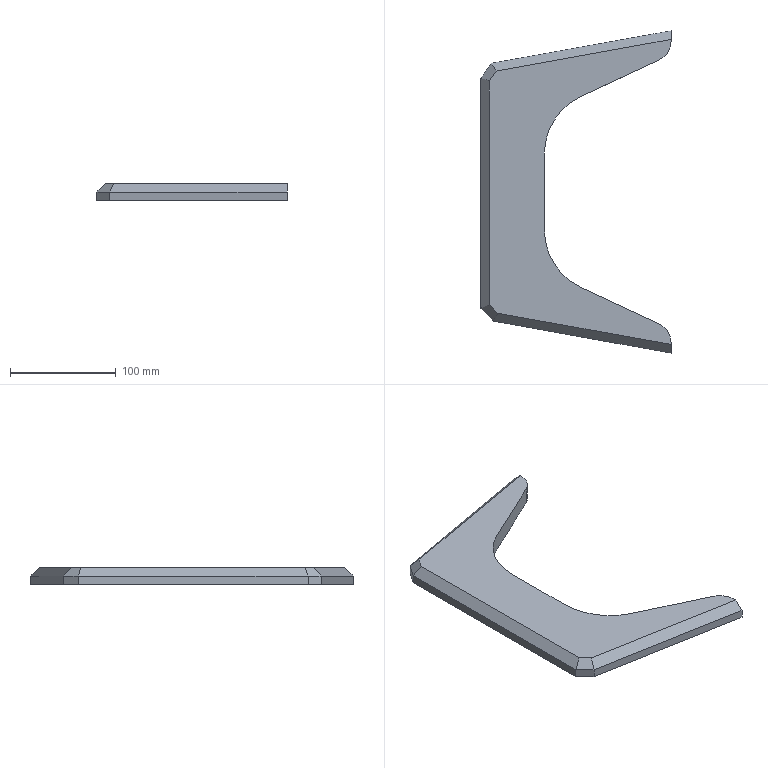Part | SolidWorks | features Chamfer 2, Extrusion 1 | 1 solid | 21 faces | box 180 x 305.1 x 16 mm | volume 379502 mm3 | plane 17 | cylinder 4 | commonest cylinder face diameters 40 x2 120 x2
STEP:
#1=CARTESIAN_POINT('',(9.84,121.779,0.));
#2=VERTEX_POINT('',#1);
#3=CARTESIAN_POINT('',(9.84,121.779,8.));
#4=VERTEX_POINT('',#3);
#5=CARTESIAN_POINT('',(9.84,121.779,16.));
#6=DIRECTION('',(0.,0.,1.));
#7=VECTOR('',#6,1000.);
#8=LINE('',#5,#7);
#9=EDGE_CURVE('',#2,#4,#8,.T.);
#10=ORIENTED_EDGE('',*,*,#9,.T.);
#11=CARTESIAN_POINT('',(180.,152.55,8.));
#12=VERTEX_POINT('',#11);
#13=CARTESIAN_POINT('',(0.,120.,8.));
#14=DIRECTION('',(0.984,0.1779,0.));
#15=VECTOR('',#14,1000.);
#16=LINE('',#13,#15);
#17=EDGE_CURVE('',#4,#12,#16,.T.);
#18=ORIENTED_EDGE('',*,*,#17,.T.);
#19=CARTESIAN_POINT('',(180.,152.55,0.));
#20=VERTEX_POINT('',#19);
#21=CARTESIAN_POINT('',(180.,152.55,16.));
#22=DIRECTION('',(0.,0.,-1.));
#23=VECTOR('',#22,1000.);
#24=LINE('',#21,#23);
#25=EDGE_CURVE('',#12,#20,#24,.T.);
#26=ORIENTED_EDGE('',*,*,#25,.T.);
#27=CARTESIAN_POINT('',(0.,120.,0.));
#28=DIRECTION('',(-0.984,-0.1779,0.));
#29=VECTOR('',#28,1000.);
#30=LINE('',#27,#29);
#31=EDGE_CURVE('',#20,#2,#30,.T.);
#32=ORIENTED_EDGE('',*,*,#31,.T.);
#33=EDGE_LOOP('',(#10,#18,#26,#32));
#34=FACE_OUTER_BOUND('',#33,.T.);
#35=CARTESIAN_POINT('',(0.,120.,16.));
#36=DIRECTION('',(0.1779,-0.984,0.));
#37=DIRECTION('',(0.984,0.1779,0.));
#38=AXIS2_PLACEMENT_3D('',#35,#36,#37);
#39=PLANE('',#38);
#40=ADVANCED_FACE('',(#34),#39,.F.);
#41=CARTESIAN_POINT('',(0.,-110.,0.));
#42=VERTEX_POINT('',#41);
#43=CARTESIAN_POINT('',(0.,-110.,8.));
#44=VERTEX_POINT('',#43);
#45=CARTESIAN_POINT('',(0.,-110.,16.));
#46=DIRECTION('',(0.,0.,1.));
#47=VECTOR('',#46,1000.);
#48=LINE('',#45,#47);
#49=EDGE_CURVE('',#42,#44,#48,.T.);
#50=ORIENTED_EDGE('',*,*,#49,.T.);
#51=CARTESIAN_POINT('',(0.,107.594,8.));
#52=VERTEX_POINT('',#51);
#53=CARTESIAN_POINT('',(0.,-120.,8.));
#54=DIRECTION('',(0.,1.,0.));
#55=VECTOR('',#54,1000.);
#56=LINE('',#53,#55);
#57=EDGE_CURVE('',#44,#52,#56,.T.);
#58=ORIENTED_EDGE('',*,*,#57,.T.);
#59=CARTESIAN_POINT('',(0.,107.594,0.));
#60=VERTEX_POINT('',#59);
#61=CARTESIAN_POINT('',(0.,107.594,16.));
#62=DIRECTION('',(0.,0.,-1.));
#63=VECTOR('',#62,1000.);
#64=LINE('',#61,#63);
#65=EDGE_CURVE('',#52,#60,#64,.T.);
#66=ORIENTED_EDGE('',*,*,#65,.T.);
#67=CARTESIAN_POINT('',(0.,-120.,0.));
#68=DIRECTION('',(0.,-1.,0.));
#69=VECTOR('',#68,1000.);
#70=LINE('',#67,#69);
#71=EDGE_CURVE('',#60,#42,#70,.T.);
#72=ORIENTED_EDGE('',*,*,#71,.T.);
#73=EDGE_LOOP('',(#50,#58,#66,#72));
#74=FACE_OUTER_BOUND('',#73,.T.);
#75=CARTESIAN_POINT('',(0.,-120.,16.));
#76=DIRECTION('',(1.,0.,0.));
#77=DIRECTION('',(0.,0.,-1.));
#78=AXIS2_PLACEMENT_3D('',#75,#76,#77);
#79=PLANE('',#78);
#80=ADVANCED_FACE('',(#74),#79,.F.);
#81=CARTESIAN_POINT('',(180.,-152.55,8.));
#82=VERTEX_POINT('',#81);
#83=CARTESIAN_POINT('',(180.,-152.55,0.));
#84=VERTEX_POINT('',#83);
#85=CARTESIAN_POINT('',(180.,-152.55,16.));
#86=DIRECTION('',(0.,0.,-1.));
#87=VECTOR('',#86,1000.);
#88=LINE('',#85,#87);
#89=EDGE_CURVE('',#82,#84,#88,.T.);
#90=ORIENTED_EDGE('',*,*,#89,.F.);
#91=CARTESIAN_POINT('',(12.208,-122.208,8.));
#92=VERTEX_POINT('',#91);
#93=CARTESIAN_POINT('',(180.,-152.55,8.));
#94=DIRECTION('',(-0.984,0.1779,0.));
#95=VECTOR('',#94,1000.);
#96=LINE('',#93,#95);
#97=EDGE_CURVE('',#82,#92,#96,.T.);
#98=ORIENTED_EDGE('',*,*,#97,.T.);
#99=CARTESIAN_POINT('',(12.208,-122.208,0.));
#100=VERTEX_POINT('',#99);
#101=CARTESIAN_POINT('',(12.208,-122.208,16.));
#102=DIRECTION('',(0.,0.,-1.));
#103=VECTOR('',#102,1000.);
#104=LINE('',#101,#103);
#105=EDGE_CURVE('',#92,#100,#104,.T.);
#106=ORIENTED_EDGE('',*,*,#105,.T.);
#107=CARTESIAN_POINT('',(180.,-152.55,0.));
#108=DIRECTION('',(0.984,-0.1779,0.));
#109=VECTOR('',#108,1000.);
#110=LINE('',#107,#109);
#111=EDGE_CURVE('',#100,#84,#110,.T.);
#112=ORIENTED_EDGE('',*,*,#111,.T.);
#113=EDGE_LOOP('',(#90,#98,#106,#112));
#114=FACE_OUTER_BOUND('',#113,.T.);
#115=CARTESIAN_POINT('',(180.,-152.55,16.));
#116=DIRECTION('',(0.1779,0.984,0.));
#117=DIRECTION('',(-0.984,0.1779,0.));
#118=AXIS2_PLACEMENT_3D('',#115,#116,#117);
#119=PLANE('',#118);
#120=ADVANCED_FACE('',(#114),#119,.F.);
#121=CARTESIAN_POINT('',(180.,-144.42,16.));
#122=VERTEX_POINT('',#121);
#123=CARTESIAN_POINT('',(180.,-142.764,16.));
#124=VERTEX_POINT('',#123);
#125=CARTESIAN_POINT('',(180.,-142.764,16.));
#126=DIRECTION('',(0.,1.,0.));
#127=VECTOR('',#126,1000.);
#128=LINE('',#125,#127);
#129=EDGE_CURVE('',#122,#124,#128,.T.);
#130=ORIENTED_EDGE('',*,*,#129,.F.);
#131=CARTESIAN_POINT('',(180.,-138.019,22.299));
#132=DIRECTION('',(0.,-0.7128,-0.7014));
#133=VECTOR('',#132,1000.);
#134=LINE('',#131,#133);
#135=EDGE_CURVE('',#122,#82,#134,.T.);
#136=ORIENTED_EDGE('',*,*,#135,.T.);
#137=ORIENTED_EDGE('',*,*,#89,.T.);
#138=CARTESIAN_POINT('',(180.,-142.764,0.));
#139=VERTEX_POINT('',#138);
#140=CARTESIAN_POINT('',(180.,-142.764,0.));
#141=DIRECTION('',(0.,1.,0.));
#142=VECTOR('',#141,1000.);
#143=LINE('',#140,#142);
#144=EDGE_CURVE('',#84,#139,#143,.T.);
#145=ORIENTED_EDGE('',*,*,#144,.T.);
#146=CARTESIAN_POINT('',(180.,-142.764,16.));
#147=DIRECTION('',(0.,0.,-1.));
#148=VECTOR('',#147,1000.);
#149=LINE('',#146,#148);
#150=EDGE_CURVE('',#124,#139,#149,.T.);
#151=ORIENTED_EDGE('',*,*,#150,.F.);
#152=EDGE_LOOP('',(#130,#136,#137,#145,#151));
#153=FACE_OUTER_BOUND('',#152,.T.);
#154=CARTESIAN_POINT('',(180.,-142.764,16.));
#155=DIRECTION('',(-1.,0.,0.));
#156=DIRECTION('',(0.,0.,1.));
#157=AXIS2_PLACEMENT_3D('',#154,#155,#156);
#158=PLANE('',#157);
#159=ADVANCED_FACE('',(#153),#158,.F.);
#160=CARTESIAN_POINT('',(168.468,-124.645,0.));
#161=VERTEX_POINT('',#160);
#162=CARTESIAN_POINT('',(160.,-142.764,0.));
#163=DIRECTION('',(0.,0.,1.));
#164=DIRECTION('',(1.,0.,0.));
#165=AXIS2_PLACEMENT_3D('',#162,#163,#164);
#166=CIRCLE('',#165,20.);
#167=EDGE_CURVE('',#139,#161,#166,.T.);
#168=ORIENTED_EDGE('',*,*,#167,.T.);
#169=CARTESIAN_POINT('',(168.468,-124.645,16.));
#170=VERTEX_POINT('',#169);
#171=CARTESIAN_POINT('',(168.468,-124.645,16.));
#172=DIRECTION('',(0.,0.,-1.));
#173=VECTOR('',#172,1000.);
#174=LINE('',#171,#173);
#175=EDGE_CURVE('',#170,#161,#174,.T.);
#176=ORIENTED_EDGE('',*,*,#175,.F.);
#177=CARTESIAN_POINT('',(160.,-142.764,16.));
#178=DIRECTION('',(0.,0.,1.));
#179=DIRECTION('',(1.,0.,0.));
#180=AXIS2_PLACEMENT_3D('',#177,#178,#179);
#181=CIRCLE('',#180,20.);
#182=EDGE_CURVE('',#124,#170,#181,.T.);
#183=ORIENTED_EDGE('',*,*,#182,.F.);
#184=ORIENTED_EDGE('',*,*,#150,.T.);
#185=EDGE_LOOP('',(#168,#176,#183,#184));
#186=FACE_OUTER_BOUND('',#185,.T.);
#187=CARTESIAN_POINT('',(160.,-142.764,16.));
#188=DIRECTION('',(0.,0.,-1.));
#189=DIRECTION('',(-1.,0.,0.));
#190=AXIS2_PLACEMENT_3D('',#187,#188,#189);
#191=CYLINDRICAL_SURFACE('',#190,20.);
#192=ADVANCED_FACE('',(#186),#191,.T.);
#193=CARTESIAN_POINT('',(94.595,-90.119,0.));
#194=VERTEX_POINT('',#193);
#195=CARTESIAN_POINT('',(94.595,-90.119,0.));
#196=DIRECTION('',(-0.9059,0.4234,0.));
#197=VECTOR('',#196,1000.);
#198=LINE('',#195,#197);
#199=EDGE_CURVE('',#161,#194,#198,.T.);
#200=ORIENTED_EDGE('',*,*,#199,.T.);
#201=CARTESIAN_POINT('',(94.595,-90.119,16.));
#202=VERTEX_POINT('',#201);
#203=CARTESIAN_POINT('',(94.595,-90.119,16.));
#204=DIRECTION('',(0.,0.,-1.));
#205=VECTOR('',#204,1000.);
#206=LINE('',#203,#205);
#207=EDGE_CURVE('',#202,#194,#206,.T.);
#208=ORIENTED_EDGE('',*,*,#207,.F.);
#209=CARTESIAN_POINT('',(94.595,-90.119,16.));
#210=DIRECTION('',(-0.9059,0.4234,0.));
#211=VECTOR('',#210,1000.);
#212=LINE('',#209,#211);
#213=EDGE_CURVE('',#170,#202,#212,.T.);
#214=ORIENTED_EDGE('',*,*,#213,.F.);
#215=ORIENTED_EDGE('',*,*,#175,.T.);
#216=EDGE_LOOP('',(#200,#208,#214,#215));
#217=FACE_OUTER_BOUND('',#216,.T.);
#218=CARTESIAN_POINT('',(94.595,-90.119,16.));
#219=DIRECTION('',(-0.4234,-0.9059,0.));
#220=DIRECTION('',(0.9059,-0.4234,0.));
#221=AXIS2_PLACEMENT_3D('',#218,#219,#220);
#222=PLANE('',#221);
#223=ADVANCED_FACE('',(#217),#222,.F.);
#224=CARTESIAN_POINT('',(60.,-35.763,0.));
#225=VERTEX_POINT('',#224);
#226=CARTESIAN_POINT('',(120.,-35.763,0.));
#227=DIRECTION('',(0.,0.,-1.));
#228=DIRECTION('',(-1.,0.,0.));
#229=AXIS2_PLACEMENT_3D('',#226,#227,#228);
#230=CIRCLE('',#229,60.);
#231=EDGE_CURVE('',#194,#225,#230,.T.);
#232=ORIENTED_EDGE('',*,*,#231,.T.);
#233=CARTESIAN_POINT('',(60.,-35.763,16.));
#234=VERTEX_POINT('',#233);
#235=CARTESIAN_POINT('',(60.,-35.763,16.));
#236=DIRECTION('',(0.,0.,-1.));
#237=VECTOR('',#236,1000.);
#238=LINE('',#235,#237);
#239=EDGE_CURVE('',#234,#225,#238,.T.);
#240=ORIENTED_EDGE('',*,*,#239,.F.);
#241=CARTESIAN_POINT('',(120.,-35.763,16.));
#242=DIRECTION('',(0.,0.,-1.));
#243=DIRECTION('',(-1.,0.,0.));
#244=AXIS2_PLACEMENT_3D('',#241,#242,#243);
#245=CIRCLE('',#244,60.);
#246=EDGE_CURVE('',#202,#234,#245,.T.);
#247=ORIENTED_EDGE('',*,*,#246,.F.);
#248=ORIENTED_EDGE('',*,*,#207,.T.);
#249=EDGE_LOOP('',(#232,#240,#247,#248));
#250=FACE_OUTER_BOUND('',#249,.T.);
#251=CARTESIAN_POINT('',(120.,-35.763,16.));
#252=DIRECTION('',(0.,0.,-1.));
#253=DIRECTION('',(-1.,0.,0.));
#254=AXIS2_PLACEMENT_3D('',#251,#252,#253);
#255=CYLINDRICAL_SURFACE('',#254,60.);
#256=ADVANCED_FACE('',(#250),#255,.F.);
#257=CARTESIAN_POINT('',(60.,35.863,0.));
#258=VERTEX_POINT('',#257);
#259=CARTESIAN_POINT('',(60.,35.863,0.));
#260=DIRECTION('',(0.,1.,0.));
#261=VECTOR('',#260,1000.);
#262=LINE('',#259,#261);
#263=EDGE_CURVE('',#225,#258,#262,.T.);
#264=ORIENTED_EDGE('',*,*,#263,.T.);
#265=CARTESIAN_POINT('',(60.,35.863,16.));
#266=VERTEX_POINT('',#265);
#267=CARTESIAN_POINT('',(60.,35.863,16.));
#268=DIRECTION('',(0.,0.,-1.));
#269=VECTOR('',#268,1000.);
#270=LINE('',#267,#269);
#271=EDGE_CURVE('',#266,#258,#270,.T.);
#272=ORIENTED_EDGE('',*,*,#271,.F.);
#273=CARTESIAN_POINT('',(60.,35.863,16.));
#274=DIRECTION('',(0.,1.,0.));
#275=VECTOR('',#274,1000.);
#276=LINE('',#273,#275);
#277=EDGE_CURVE('',#234,#266,#276,.T.);
#278=ORIENTED_EDGE('',*,*,#277,.F.);
#279=ORIENTED_EDGE('',*,*,#239,.T.);
#280=EDGE_LOOP('',(#264,#272,#278,#279));
#281=FACE_OUTER_BOUND('',#280,.T.);
#282=CARTESIAN_POINT('',(60.,35.863,16.));
#283=DIRECTION('',(-1.,0.,0.));
#284=DIRECTION('',(0.,0.,1.));
#285=AXIS2_PLACEMENT_3D('',#282,#283,#284);
#286=PLANE('',#285);
#287=ADVANCED_FACE('',(#281),#286,.F.);
#288=CARTESIAN_POINT('',(94.595,90.219,0.));
#289=VERTEX_POINT('',#288);
#290=CARTESIAN_POINT('',(120.,35.863,0.));
#291=DIRECTION('',(0.,0.,-1.));
#292=DIRECTION('',(-1.,0.,0.));
#293=AXIS2_PLACEMENT_3D('',#290,#291,#292);
#294=CIRCLE('',#293,60.);
#295=EDGE_CURVE('',#258,#289,#294,.T.);
#296=ORIENTED_EDGE('',*,*,#295,.T.);
#297=CARTESIAN_POINT('',(94.595,90.219,16.));
#298=VERTEX_POINT('',#297);
#299=CARTESIAN_POINT('',(94.595,90.219,16.));
#300=DIRECTION('',(0.,0.,-1.));
#301=VECTOR('',#300,1000.);
#302=LINE('',#299,#301);
#303=EDGE_CURVE('',#298,#289,#302,.T.);
#304=ORIENTED_EDGE('',*,*,#303,.F.);
#305=CARTESIAN_POINT('',(120.,35.863,16.));
#306=DIRECTION('',(0.,0.,-1.));
#307=DIRECTION('',(-1.,0.,0.));
#308=AXIS2_PLACEMENT_3D('',#305,#306,#307);
#309=CIRCLE('',#308,60.);
#310=EDGE_CURVE('',#266,#298,#309,.T.);
#311=ORIENTED_EDGE('',*,*,#310,.F.);
#312=ORIENTED_EDGE('',*,*,#271,.T.);
#313=EDGE_LOOP('',(#296,#304,#311,#312));
#314=FACE_OUTER_BOUND('',#313,.T.);
#315=CARTESIAN_POINT('',(120.,35.863,16.));
#316=DIRECTION('',(0.,0.,-1.));
#317=DIRECTION('',(-1.,0.,0.));
#318=AXIS2_PLACEMENT_3D('',#315,#316,#317);
#319=CYLINDRICAL_SURFACE('',#318,60.);
#320=ADVANCED_FACE('',(#314),#319,.F.);
#321=CARTESIAN_POINT('',(168.468,124.745,0.));
#322=VERTEX_POINT('',#321);
#323=CARTESIAN_POINT('',(168.468,124.745,0.));
#324=DIRECTION('',(0.9059,0.4234,0.));
#325=VECTOR('',#324,1000.);
#326=LINE('',#323,#325);
#327=EDGE_CURVE('',#289,#322,#326,.T.);
#328=ORIENTED_EDGE('',*,*,#327,.T.);
#329=CARTESIAN_POINT('',(168.468,124.745,16.));
#330=VERTEX_POINT('',#329);
#331=CARTESIAN_POINT('',(168.468,124.745,16.));
#332=DIRECTION('',(0.,0.,-1.));
#333=VECTOR('',#332,1000.);
#334=LINE('',#331,#333);
#335=EDGE_CURVE('',#330,#322,#334,.T.);
#336=ORIENTED_EDGE('',*,*,#335,.F.);
#337=CARTESIAN_POINT('',(168.468,124.745,16.));
#338=DIRECTION('',(0.9059,0.4234,0.));
#339=VECTOR('',#338,1000.);
#340=LINE('',#337,#339);
#341=EDGE_CURVE('',#298,#330,#340,.T.);
#342=ORIENTED_EDGE('',*,*,#341,.F.);
#343=ORIENTED_EDGE('',*,*,#303,.T.);
#344=EDGE_LOOP('',(#328,#336,#342,#343));
#345=FACE_OUTER_BOUND('',#344,.T.);
#346=CARTESIAN_POINT('',(168.468,124.745,16.));
#347=DIRECTION('',(-0.4234,0.9059,0.));
#348=DIRECTION('',(-0.9059,-0.4234,0.));
#349=AXIS2_PLACEMENT_3D('',#346,#347,#348);
#350=PLANE('',#349);
#351=ADVANCED_FACE('',(#345),#350,.F.);
#352=CARTESIAN_POINT('',(180.,142.864,0.));
#353=VERTEX_POINT('',#352);
#354=CARTESIAN_POINT('',(160.,142.864,0.));
#355=DIRECTION('',(0.,0.,1.));
#356=DIRECTION('',(-1.,0.,0.));
#357=AXIS2_PLACEMENT_3D('',#354,#355,#356);
#358=CIRCLE('',#357,20.);
#359=EDGE_CURVE('',#322,#353,#358,.T.);
#360=ORIENTED_EDGE('',*,*,#359,.T.);
#361=CARTESIAN_POINT('',(180.,142.864,16.));
#362=VERTEX_POINT('',#361);
#363=CARTESIAN_POINT('',(180.,142.864,16.));
#364=DIRECTION('',(0.,0.,-1.));
#365=VECTOR('',#364,1000.);
#366=LINE('',#363,#365);
#367=EDGE_CURVE('',#362,#353,#366,.T.);
#368=ORIENTED_EDGE('',*,*,#367,.F.);
#369=CARTESIAN_POINT('',(160.,142.864,16.));
#370=DIRECTION('',(0.,0.,1.));
#371=DIRECTION('',(-1.,0.,0.));
#372=AXIS2_PLACEMENT_3D('',#369,#370,#371);
#373=CIRCLE('',#372,20.);
#374=EDGE_CURVE('',#330,#362,#373,.T.);
#375=ORIENTED_EDGE('',*,*,#374,.F.);
#376=ORIENTED_EDGE('',*,*,#335,.T.);
#377=EDGE_LOOP('',(#360,#368,#375,#376));
#378=FACE_OUTER_BOUND('',#377,.T.);
#379=CARTESIAN_POINT('',(160.,142.864,16.));
#380=DIRECTION('',(0.,0.,-1.));
#381=DIRECTION('',(-1.,0.,0.));
#382=AXIS2_PLACEMENT_3D('',#379,#380,#381);
#383=CYLINDRICAL_SURFACE('',#382,20.);
#384=ADVANCED_FACE('',(#378),#383,.T.);
#385=ORIENTED_EDGE('',*,*,#25,.F.);
#386=CARTESIAN_POINT('',(180.,144.42,16.));
#387=VERTEX_POINT('',#386);
#388=CARTESIAN_POINT('',(180.,142.616,17.775));
#389=DIRECTION('',(0.,-0.7128,0.7014));
#390=VECTOR('',#389,1000.);
#391=LINE('',#388,#390);
#392=EDGE_CURVE('',#12,#387,#391,.T.);
#393=ORIENTED_EDGE('',*,*,#392,.T.);
#394=CARTESIAN_POINT('',(180.,152.55,16.));
#395=DIRECTION('',(0.,1.,0.));
#396=VECTOR('',#395,1000.);
#397=LINE('',#394,#396);
#398=EDGE_CURVE('',#362,#387,#397,.T.);
#399=ORIENTED_EDGE('',*,*,#398,.F.);
#400=ORIENTED_EDGE('',*,*,#367,.T.);
#401=CARTESIAN_POINT('',(180.,152.55,0.));
#402=DIRECTION('',(0.,1.,0.));
#403=VECTOR('',#402,1000.);
#404=LINE('',#401,#403);
#405=EDGE_CURVE('',#353,#20,#404,.T.);
#406=ORIENTED_EDGE('',*,*,#405,.T.);
#407=EDGE_LOOP('',(#385,#393,#399,#400,#406));
#408=FACE_OUTER_BOUND('',#407,.T.);
#409=CARTESIAN_POINT('',(180.,152.55,16.));
#410=DIRECTION('',(-1.,0.,0.));
#411=DIRECTION('',(0.,-1.,0.));
#412=AXIS2_PLACEMENT_3D('',#409,#410,#411);
#413=PLANE('',#412);
#414=ADVANCED_FACE('',(#408),#413,.F.);
#415=ORIENTED_EDGE('',*,*,#398,.T.);
#416=CARTESIAN_POINT('',(14.525,114.497,16.));
#417=VERTEX_POINT('',#416);
#418=CARTESIAN_POINT('',(160.361,140.869,16.));
#419=DIRECTION('',(-0.984,-0.1779,0.));
#420=VECTOR('',#419,1000.);
#421=LINE('',#418,#420);
#422=EDGE_CURVE('',#387,#417,#421,.T.);
#423=ORIENTED_EDGE('',*,*,#422,.T.);
#424=CARTESIAN_POINT('',(8.,105.091,16.));
#425=VERTEX_POINT('',#424);
#426=CARTESIAN_POINT('',(6.573,103.035,16.));
#427=DIRECTION('',(-0.57,-0.8216,0.));
#428=VECTOR('',#427,1000.);
#429=LINE('',#426,#428);
#430=EDGE_CURVE('',#417,#425,#429,.T.);
#431=ORIENTED_EDGE('',*,*,#430,.T.);
#432=CARTESIAN_POINT('',(8.,-106.686,16.));
#433=VERTEX_POINT('',#432);
#434=CARTESIAN_POINT('',(8.,142.864,16.));
#435=DIRECTION('',(0.,-1.,0.));
#436=VECTOR('',#435,1000.);
#437=LINE('',#434,#436);
#438=EDGE_CURVE('',#425,#433,#437,.T.);
#439=ORIENTED_EDGE('',*,*,#438,.T.);
#440=CARTESIAN_POINT('',(16.094,-114.781,16.));
#441=VERTEX_POINT('',#440);
#442=CARTESIAN_POINT('',(17.864,-116.551,16.));
#443=DIRECTION('',(0.7071,-0.7071,0.));
#444=VECTOR('',#443,1000.);
#445=LINE('',#442,#444);
#446=EDGE_CURVE('',#433,#441,#445,.T.);
#447=ORIENTED_EDGE('',*,*,#446,.T.);
#448=CARTESIAN_POINT('',(110.328,-131.821,16.));
#449=DIRECTION('',(0.984,-0.1779,0.));
#450=VECTOR('',#449,1000.);
#451=LINE('',#448,#450);
#452=EDGE_CURVE('',#441,#122,#451,.T.);
#453=ORIENTED_EDGE('',*,*,#452,.T.);
#454=ORIENTED_EDGE('',*,*,#129,.T.);
#455=ORIENTED_EDGE('',*,*,#182,.T.);
#456=ORIENTED_EDGE('',*,*,#213,.T.);
#457=ORIENTED_EDGE('',*,*,#246,.T.);
#458=ORIENTED_EDGE('',*,*,#277,.T.);
#459=ORIENTED_EDGE('',*,*,#310,.T.);
#460=ORIENTED_EDGE('',*,*,#341,.T.);
#461=ORIENTED_EDGE('',*,*,#374,.T.);
#462=EDGE_LOOP('',(#415,#423,#431,#439,#447,#453,#454,#455,#456,#457,#458,#459,#460,#461));
#463=FACE_OUTER_BOUND('',#462,.T.);
#464=CARTESIAN_POINT('',(160.,142.864,16.));
#465=DIRECTION('',(0.,0.,-1.));
#466=DIRECTION('',(-1.,0.,0.));
#467=AXIS2_PLACEMENT_3D('',#464,#465,#466);
#468=PLANE('',#467);
#469=ADVANCED_FACE('',(#463),#468,.F.);
#470=ORIENTED_EDGE('',*,*,#71,.F.);
#471=CARTESIAN_POINT('',(68.501,206.339,0.));
#472=DIRECTION('',(0.57,0.8216,0.));
#473=VECTOR('',#472,1000.);
#474=LINE('',#471,#473);
#475=EDGE_CURVE('',#60,#2,#474,.T.);
#476=ORIENTED_EDGE('',*,*,#475,.T.);
#477=ORIENTED_EDGE('',*,*,#31,.F.);
#478=ORIENTED_EDGE('',*,*,#405,.F.);
#479=ORIENTED_EDGE('',*,*,#359,.F.);
#480=ORIENTED_EDGE('',*,*,#327,.F.);
#481=ORIENTED_EDGE('',*,*,#295,.F.);
#482=ORIENTED_EDGE('',*,*,#263,.F.);
#483=ORIENTED_EDGE('',*,*,#231,.F.);
#484=ORIENTED_EDGE('',*,*,#199,.F.);
#485=ORIENTED_EDGE('',*,*,#167,.F.);
#486=ORIENTED_EDGE('',*,*,#144,.F.);
#487=ORIENTED_EDGE('',*,*,#111,.F.);
#488=CARTESIAN_POINT('',(-46.432,-63.568,0.));
#489=DIRECTION('',(-0.7071,0.7071,0.));
#490=VECTOR('',#489,1000.);
#491=LINE('',#488,#490);
#492=EDGE_CURVE('',#100,#42,#491,.T.);
#493=ORIENTED_EDGE('',*,*,#492,.T.);
#494=EDGE_LOOP('',(#470,#476,#477,#478,#479,#480,#481,#482,#483,#484,#485,#486,#487,#493));
#495=FACE_OUTER_BOUND('',#494,.T.);
#496=CARTESIAN_POINT('',(160.,142.864,0.));
#497=DIRECTION('',(0.,0.,-1.));
#498=DIRECTION('',(-1.,0.,0.));
#499=AXIS2_PLACEMENT_3D('',#496,#497,#498);
#500=PLANE('',#499);
#501=ADVANCED_FACE('',(#495),#500,.T.);
#502=ORIENTED_EDGE('',*,*,#65,.F.);
#503=CARTESIAN_POINT('',(9.84,121.779,8.));
#504=DIRECTION('',(0.57,0.8216,0.));
#505=VECTOR('',#504,1000.);
#506=LINE('',#503,#505);
#507=EDGE_CURVE('',#52,#4,#506,.T.);
#508=ORIENTED_EDGE('',*,*,#507,.T.);
#509=ORIENTED_EDGE('',*,*,#9,.F.);
#510=ORIENTED_EDGE('',*,*,#475,.F.);
#511=EDGE_LOOP('',(#502,#508,#509,#510));
#512=FACE_OUTER_BOUND('',#511,.T.);
#513=CARTESIAN_POINT('',(0.,107.594,16.));
#514=DIRECTION('',(0.8216,-0.57,0.));
#515=DIRECTION('',(0.57,0.8216,0.));
#516=AXIS2_PLACEMENT_3D('',#513,#514,#515);
#517=PLANE('',#516);
#518=ADVANCED_FACE('',(#512),#517,.F.);
#519=ORIENTED_EDGE('',*,*,#105,.F.);
#520=CARTESIAN_POINT('',(0.,-110.,8.));
#521=DIRECTION('',(-0.7071,0.7071,0.));
#522=VECTOR('',#521,1000.);
#523=LINE('',#520,#522);
#524=EDGE_CURVE('',#92,#44,#523,.T.);
#525=ORIENTED_EDGE('',*,*,#524,.T.);
#526=ORIENTED_EDGE('',*,*,#49,.F.);
#527=ORIENTED_EDGE('',*,*,#492,.F.);
#528=EDGE_LOOP('',(#519,#525,#526,#527));
#529=FACE_OUTER_BOUND('',#528,.T.);
#530=CARTESIAN_POINT('',(12.208,-122.208,16.));
#531=DIRECTION('',(0.7071,0.7071,0.));
#532=DIRECTION('',(-0.7071,0.7071,0.));
#533=AXIS2_PLACEMENT_3D('',#530,#531,#532);
#534=PLANE('',#533);
#535=ADVANCED_FACE('',(#529),#534,.F.);
#536=ORIENTED_EDGE('',*,*,#135,.F.);
#537=ORIENTED_EDGE('',*,*,#452,.F.);
#538=CARTESIAN_POINT('',(23.034,-101.521,30.283));
#539=DIRECTION('',(0.3354,0.6409,0.6904));
#540=VECTOR('',#539,1000.);
#541=LINE('',#538,#540);
#542=EDGE_CURVE('',#92,#441,#541,.T.);
#543=ORIENTED_EDGE('',*,*,#542,.F.);
#544=ORIENTED_EDGE('',*,*,#97,.F.);
#545=EDGE_LOOP('',(#536,#537,#543,#544));
#546=FACE_OUTER_BOUND('',#545,.T.);
#547=CARTESIAN_POINT('',(110.328,-131.821,16.));
#548=DIRECTION('',(0.1258,0.6958,-0.7071));
#549=DIRECTION('',(0.,0.7128,0.7014));
#550=AXIS2_PLACEMENT_3D('',#547,#548,#549);
#551=PLANE('',#550);
#552=ADVANCED_FACE('',(#546),#551,.F.);
#553=ORIENTED_EDGE('',*,*,#542,.T.);
#554=ORIENTED_EDGE('',*,*,#446,.F.);
#555=CARTESIAN_POINT('',(-5.157,-112.136,2.843));
#556=DIRECTION('',(0.6786,0.2811,0.6786));
#557=VECTOR('',#556,1000.);
#558=LINE('',#555,#557);
#559=EDGE_CURVE('',#44,#433,#558,.T.);
#560=ORIENTED_EDGE('',*,*,#559,.F.);
#561=ORIENTED_EDGE('',*,*,#524,.F.);
#562=EDGE_LOOP('',(#553,#554,#560,#561));
#563=FACE_OUTER_BOUND('',#562,.T.);
#564=CARTESIAN_POINT('',(-40.775,-57.911,16.));
#565=DIRECTION('',(0.5,0.5,-0.7071));
#566=DIRECTION('',(-0.8165,0.,-0.5774));
#567=AXIS2_PLACEMENT_3D('',#564,#565,#566);
#568=PLANE('',#567);
#569=ADVANCED_FACE('',(#563),#568,.F.);
#570=ORIENTED_EDGE('',*,*,#559,.T.);
#571=ORIENTED_EDGE('',*,*,#438,.F.);
#572=CARTESIAN_POINT('',(2.366,106.854,10.366));
#573=DIRECTION('',(0.6904,-0.216,0.6904));
#574=VECTOR('',#573,1000.);
#575=LINE('',#572,#574);
#576=EDGE_CURVE('',#52,#425,#575,.T.);
#577=ORIENTED_EDGE('',*,*,#576,.F.);
#578=ORIENTED_EDGE('',*,*,#57,.F.);
#579=EDGE_LOOP('',(#570,#571,#577,#578));
#580=FACE_OUTER_BOUND('',#579,.T.);
#581=CARTESIAN_POINT('',(8.,142.864,16.));
#582=DIRECTION('',(0.7071,0.,-0.7071));
#583=DIRECTION('',(-0.7071,0.,-0.7071));
#584=AXIS2_PLACEMENT_3D('',#581,#582,#583);
#585=PLANE('',#584);
#586=ADVANCED_FACE('',(#580),#585,.F.);
#587=ORIENTED_EDGE('',*,*,#576,.T.);
#588=ORIENTED_EDGE('',*,*,#430,.F.);
#589=CARTESIAN_POINT('',(2.66,132.942,-4.262));
#590=DIRECTION('',(0.3974,-0.6177,0.6786));
#591=VECTOR('',#590,1000.);
#592=LINE('',#589,#591);
#593=EDGE_CURVE('',#4,#417,#592,.T.);
#594=ORIENTED_EDGE('',*,*,#593,.F.);
#595=ORIENTED_EDGE('',*,*,#507,.F.);
#596=EDGE_LOOP('',(#587,#588,#594,#595));
#597=FACE_OUTER_BOUND('',#596,.T.);
#598=CARTESIAN_POINT('',(75.074,201.779,16.));
#599=DIRECTION('',(0.581,-0.403,-0.7071));
#600=DIRECTION('',(-0.7726,0.,-0.6348));
#601=AXIS2_PLACEMENT_3D('',#598,#599,#600);
#602=PLANE('',#601);
#603=ADVANCED_FACE('',(#597),#602,.F.);
#604=ORIENTED_EDGE('',*,*,#392,.F.);
#605=ORIENTED_EDGE('',*,*,#17,.F.);
#606=ORIENTED_EDGE('',*,*,#593,.T.);
#607=ORIENTED_EDGE('',*,*,#422,.F.);
#608=EDGE_LOOP('',(#604,#605,#606,#607));
#609=FACE_OUTER_BOUND('',#608,.T.);
#610=CARTESIAN_POINT('',(160.361,140.869,16.));
#611=DIRECTION('',(0.1258,-0.6958,-0.7071));
#612=DIRECTION('',(0.,0.7128,-0.7014));
#613=AXIS2_PLACEMENT_3D('',#610,#611,#612);
#614=PLANE('',#613);
#615=ADVANCED_FACE('',(#609),#614,.F.);
#616=CLOSED_SHELL('',(#40,#80,#120,#159,#192,#223,#256,#287,#320,#351,#384,#414,#469,#501,#518,#535,#552,#569,#586,#603,#615));
#617=MANIFOLD_SOLID_BREP('',#616);
#618=CARTESIAN_POINT('',(0.,0.,0.));
#619=DIRECTION('',(0.,0.,1.));
#620=DIRECTION('',(1.,0.,0.));
#621=AXIS2_PLACEMENT_3D('',#618,#619,#620);
#622=(LENGTH_UNIT()NAMED_UNIT(*)SI_UNIT(.MILLI.,.METRE.));
#623=UNCERTAINTY_MEASURE_WITH_UNIT(LENGTH_MEASURE(0.00001),#622,'','');
#624=(NAMED_UNIT(*)PLANE_ANGLE_UNIT()SI_UNIT($,.RADIAN.));
#625=(NAMED_UNIT(*)SI_UNIT($,.STERADIAN.)SOLID_ANGLE_UNIT());
#626=(GEOMETRIC_REPRESENTATION_CONTEXT(3)GLOBAL_UNCERTAINTY_ASSIGNED_CONTEXT((#623))GLOBAL_UNIT_ASSIGNED_CONTEXT((#622,#624,#625))REPRESENTATION_CONTEXT('',''));
#627=ADVANCED_BREP_SHAPE_REPRESENTATION('',(#617,#621),#626);